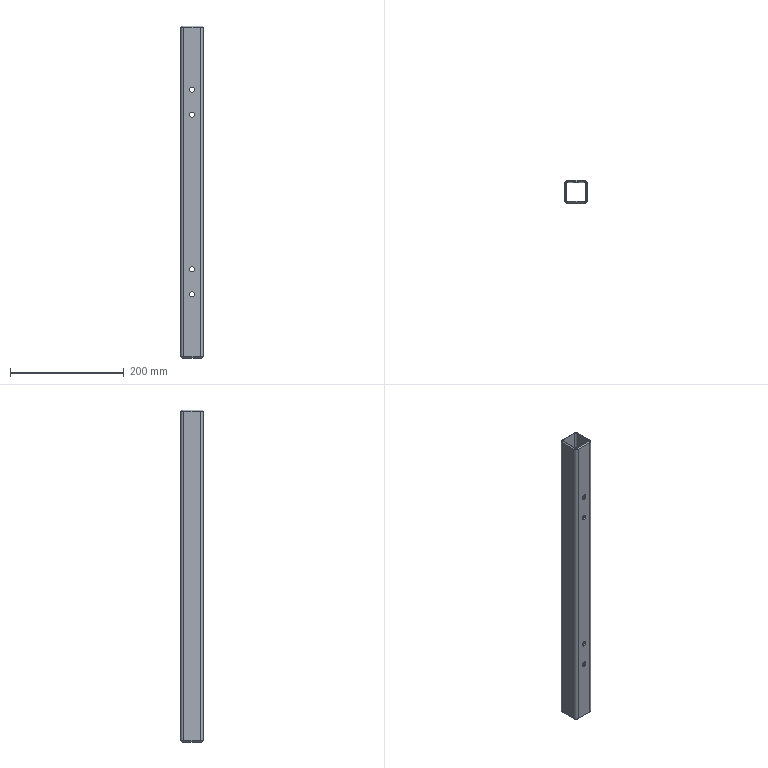Part | STEP file | IN-01-01-03-01 | 1 solid | 50 faces | box 40 x 40 x 584 mm | volume 236623 mm3 | cylinder 24 | plane 18 | cone 8 | commonest cylinder face diameters 9 x16 5.8 x4 11.6 x4